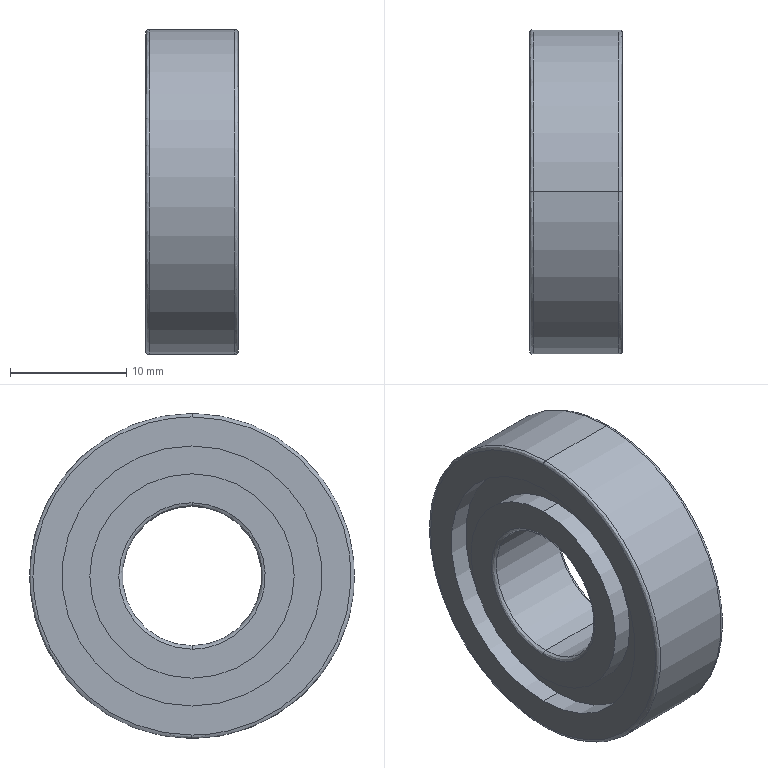Part | SolidWorks | features BaseBody 1 | 1 solid | 26 faces | box 8 x 28 x 28 mm | volume 3486 mm3 | cylinder 12 | spline 8 | plane 6 | commonest cylinder face diameters 17.6 x4 22.4 x4 12 x2 28 x2
STEP:
#1=CARTESIAN_POINT('',(0.,0.,13.7));
#2=VERTEX_POINT('',#1);
#3=CARTESIAN_POINT('',(0.,0.,-13.7));
#4=VERTEX_POINT('',#3);
#5=CARTESIAN_POINT('',(0.,0.,13.7));
#6=CARTESIAN_POINT('',(0.,-27.4,13.7));
#7=CARTESIAN_POINT('',(0.,-27.4,-13.7));
#8=CARTESIAN_POINT('',(0.,0.,-13.7));
#9=(BOUNDED_CURVE()B_SPLINE_CURVE(3,(#5,#6,#7,#8),.UNSPECIFIED.,.F.,.F.)B_SPLINE_CURVE_WITH_KNOTS((4,4),(0.,1.),.UNSPECIFIED.)CURVE()GEOMETRIC_REPRESENTATION_ITEM()RATIONAL_B_SPLINE_CURVE((1.,0.3333,0.3333,1.))REPRESENTATION_ITEM(''));
#10=EDGE_CURVE('',#2,#4,#9,.T.);
#11=ORIENTED_EDGE('',*,*,#10,.T.);
#12=CARTESIAN_POINT('',(0.3,0.,-14.));
#13=VERTEX_POINT('',#12);
#14=CARTESIAN_POINT('',(0.3,0.,-13.7));
#15=DIRECTION('',(0.,-1.,0.));
#16=DIRECTION('',(0.,0.,-1.));
#17=AXIS2_PLACEMENT_3D('',#14,#15,#16);
#18=CIRCLE('',#17,0.3);
#19=EDGE_CURVE('',#4,#13,#18,.T.);
#20=ORIENTED_EDGE('',*,*,#19,.T.);
#21=CARTESIAN_POINT('',(0.3,0.,14.));
#22=VERTEX_POINT('',#21);
#23=CARTESIAN_POINT('',(0.3,0.,0.));
#24=DIRECTION('',(1.,0.,0.));
#25=DIRECTION('',(0.,0.,-1.));
#26=AXIS2_PLACEMENT_3D('',#23,#24,#25);
#27=CIRCLE('',#26,14.);
#28=EDGE_CURVE('',#22,#13,#27,.T.);
#29=ORIENTED_EDGE('',*,*,#28,.F.);
#30=CARTESIAN_POINT('',(0.3,0.,13.7));
#31=DIRECTION('',(0.,1.,0.));
#32=DIRECTION('',(0.,0.,1.));
#33=AXIS2_PLACEMENT_3D('',#30,#31,#32);
#34=CIRCLE('',#33,0.3);
#35=EDGE_CURVE('',#2,#22,#34,.T.);
#36=ORIENTED_EDGE('',*,*,#35,.F.);
#37=EDGE_LOOP('',(#11,#20,#29,#36));
#38=FACE_OUTER_BOUND('',#37,.T.);
#39=CARTESIAN_POINT('',(0.,0.,-13.7));
#40=CARTESIAN_POINT('',(0.,-27.4,-13.7));
#41=CARTESIAN_POINT('',(0.,-27.4,13.7));
#42=CARTESIAN_POINT('',(0.,0.,13.7));
#43=CARTESIAN_POINT('',(0.,0.,-13.876));
#44=CARTESIAN_POINT('',(0.,-27.751,-13.876));
#45=CARTESIAN_POINT('',(0.,-27.751,13.876));
#46=CARTESIAN_POINT('',(0.,0.,13.876));
#47=CARTESIAN_POINT('',(0.1243,0.,-14.));
#48=CARTESIAN_POINT('',(0.1243,-28.,-14.));
#49=CARTESIAN_POINT('',(0.1243,-28.,14.));
#50=CARTESIAN_POINT('',(0.1243,0.,14.));
#51=CARTESIAN_POINT('',(0.3,0.,-14.));
#52=CARTESIAN_POINT('',(0.3,-28.,-14.));
#53=CARTESIAN_POINT('',(0.3,-28.,14.));
#54=CARTESIAN_POINT('',(0.3,0.,14.));
#55=(BOUNDED_SURFACE()B_SPLINE_SURFACE(3,3,((#39,#40,#41,#42),(#43,#44,#45,#46),(#47,#48,#49,#50),(#51,#52,#53,#54)),.UNSPECIFIED.,.F.,.F.,.F.)B_SPLINE_SURFACE_WITH_KNOTS((4,4),(4,4),(0.,1.),(0.,1.),.UNSPECIFIED.)GEOMETRIC_REPRESENTATION_ITEM()RATIONAL_B_SPLINE_SURFACE(((1.,0.3333,0.3333,1.),(0.8047,0.2682,0.2682,0.8047),(0.8047,0.2682,0.2682,0.8047),(1.,0.3333,0.3333,1.)))REPRESENTATION_ITEM('')SURFACE());
#56=ADVANCED_FACE('',(#38),#55,.T.);
#57=CARTESIAN_POINT('',(7.7,0.,-14.));
#58=VERTEX_POINT('',#57);
#59=CARTESIAN_POINT('',(7.7,0.,14.));
#60=VERTEX_POINT('',#59);
#61=CARTESIAN_POINT('',(7.7,0.,0.));
#62=DIRECTION('',(-1.,0.,0.));
#63=DIRECTION('',(0.,0.,-1.));
#64=AXIS2_PLACEMENT_3D('',#61,#62,#63);
#65=CIRCLE('',#64,14.);
#66=EDGE_CURVE('',#58,#60,#65,.T.);
#67=ORIENTED_EDGE('',*,*,#66,.F.);
#68=CARTESIAN_POINT('',(8.,0.,-13.7));
#69=VERTEX_POINT('',#68);
#70=CARTESIAN_POINT('',(7.7,0.,-13.7));
#71=DIRECTION('',(0.,-1.,0.));
#72=DIRECTION('',(0.,0.,-1.));
#73=AXIS2_PLACEMENT_3D('',#70,#71,#72);
#74=CIRCLE('',#73,0.3);
#75=EDGE_CURVE('',#58,#69,#74,.T.);
#76=ORIENTED_EDGE('',*,*,#75,.T.);
#77=CARTESIAN_POINT('',(8.,0.,13.7));
#78=VERTEX_POINT('',#77);
#79=CARTESIAN_POINT('',(8.,0.,-13.7));
#80=CARTESIAN_POINT('',(8.,-27.4,-13.7));
#81=CARTESIAN_POINT('',(8.,-27.4,13.7));
#82=CARTESIAN_POINT('',(8.,0.,13.7));
#83=(BOUNDED_CURVE()B_SPLINE_CURVE(3,(#79,#80,#81,#82),.UNSPECIFIED.,.F.,.F.)B_SPLINE_CURVE_WITH_KNOTS((4,4),(0.,1.),.UNSPECIFIED.)CURVE()GEOMETRIC_REPRESENTATION_ITEM()RATIONAL_B_SPLINE_CURVE((1.,0.3333,0.3333,1.))REPRESENTATION_ITEM(''));
#84=EDGE_CURVE('',#69,#78,#83,.T.);
#85=ORIENTED_EDGE('',*,*,#84,.T.);
#86=CARTESIAN_POINT('',(7.7,0.,13.7));
#87=DIRECTION('',(0.,1.,0.));
#88=DIRECTION('',(0.,0.,1.));
#89=AXIS2_PLACEMENT_3D('',#86,#87,#88);
#90=CIRCLE('',#89,0.3);
#91=EDGE_CURVE('',#60,#78,#90,.T.);
#92=ORIENTED_EDGE('',*,*,#91,.F.);
#93=EDGE_LOOP('',(#67,#76,#85,#92));
#94=FACE_OUTER_BOUND('',#93,.T.);
#95=CARTESIAN_POINT('',(7.7,0.,-14.));
#96=CARTESIAN_POINT('',(7.7,-28.,-14.));
#97=CARTESIAN_POINT('',(7.7,-28.,14.));
#98=CARTESIAN_POINT('',(7.7,0.,14.));
#99=CARTESIAN_POINT('',(7.876,0.,-14.));
#100=CARTESIAN_POINT('',(7.876,-28.,-14.));
#101=CARTESIAN_POINT('',(7.876,-28.,14.));
#102=CARTESIAN_POINT('',(7.876,0.,14.));
#103=CARTESIAN_POINT('',(8.,0.,-13.876));
#104=CARTESIAN_POINT('',(8.,-27.751,-13.876));
#105=CARTESIAN_POINT('',(8.,-27.751,13.876));
#106=CARTESIAN_POINT('',(8.,0.,13.876));
#107=CARTESIAN_POINT('',(8.,0.,-13.7));
#108=CARTESIAN_POINT('',(8.,-27.4,-13.7));
#109=CARTESIAN_POINT('',(8.,-27.4,13.7));
#110=CARTESIAN_POINT('',(8.,0.,13.7));
#111=(BOUNDED_SURFACE()B_SPLINE_SURFACE(3,3,((#95,#96,#97,#98),(#99,#100,#101,#102),(#103,#104,#105,#106),(#107,#108,#109,#110)),.UNSPECIFIED.,.F.,.F.,.F.)B_SPLINE_SURFACE_WITH_KNOTS((4,4),(4,4),(0.,1.),(0.,1.),.UNSPECIFIED.)GEOMETRIC_REPRESENTATION_ITEM()RATIONAL_B_SPLINE_SURFACE(((1.,0.3333,0.3333,1.),(0.8047,0.2682,0.2682,0.8047),(0.8047,0.2682,0.2682,0.8047),(1.,0.3333,0.3333,1.)))REPRESENTATION_ITEM('')SURFACE());
#112=ADVANCED_FACE('',(#94),#111,.T.);
#113=CARTESIAN_POINT('',(0.3,0.,6.));
#114=VERTEX_POINT('',#113);
#115=CARTESIAN_POINT('',(0.3,0.,-6.));
#116=VERTEX_POINT('',#115);
#117=CARTESIAN_POINT('',(0.3,0.,0.));
#118=DIRECTION('',(1.,0.,0.));
#119=DIRECTION('',(0.,0.,1.));
#120=AXIS2_PLACEMENT_3D('',#117,#118,#119);
#121=CIRCLE('',#120,6.);
#122=EDGE_CURVE('',#114,#116,#121,.T.);
#123=ORIENTED_EDGE('',*,*,#122,.T.);
#124=CARTESIAN_POINT('',(0.,0.,-6.3));
#125=VERTEX_POINT('',#124);
#126=CARTESIAN_POINT('',(0.3,0.,-6.3));
#127=DIRECTION('',(0.,-1.,0.));
#128=DIRECTION('',(0.,0.,-1.));
#129=AXIS2_PLACEMENT_3D('',#126,#127,#128);
#130=CIRCLE('',#129,0.3);
#131=EDGE_CURVE('',#116,#125,#130,.T.);
#132=ORIENTED_EDGE('',*,*,#131,.T.);
#133=CARTESIAN_POINT('',(0.,0.,6.3));
#134=VERTEX_POINT('',#133);
#135=CARTESIAN_POINT('',(0.,0.,6.3));
#136=CARTESIAN_POINT('',(0.,-0.1928,6.3));
#137=CARTESIAN_POINT('',(0.,-0.4806,6.287));
#138=CARTESIAN_POINT('',(0.,-0.8142,6.248));
#139=CARTESIAN_POINT('',(0.,-0.9805,6.224));
#140=CARTESIAN_POINT('',(0.,-1.052,6.212));
#141=CARTESIAN_POINT('',(0.,-1.099,6.203));
#142=CARTESIAN_POINT('',(0.,-1.121,6.199));
#143=CARTESIAN_POINT('',(0.,-1.347,6.158));
#144=CARTESIAN_POINT('',(0.,-1.644,6.088));
#145=CARTESIAN_POINT('',(0.,-1.984,5.981));
#146=CARTESIAN_POINT('',(0.,-2.128,5.93));
#147=CARTESIAN_POINT('',(0.,-2.224,5.895));
#148=CARTESIAN_POINT('',(0.,-2.27,5.877));
#149=CARTESIAN_POINT('',(0.,-2.517,5.779));
#150=CARTESIAN_POINT('',(0.,-2.806,5.648));
#151=CARTESIAN_POINT('',(0.,-3.085,5.494));
#152=CARTESIAN_POINT('',(0.,-3.268,5.387));
#153=CARTESIAN_POINT('',(0.,-3.356,5.333));
#154=CARTESIAN_POINT('',(0.,-3.811,5.035));
#155=CARTESIAN_POINT('',(0.,-4.147,4.762));
#156=CARTESIAN_POINT('',(0.,-4.608,4.301));
#157=CARTESIAN_POINT('',(0.,-4.826,4.06));
#158=CARTESIAN_POINT('',(0.,-5.057,3.76));
#159=CARTESIAN_POINT('',(0.,-5.151,3.627));
#160=CARTESIAN_POINT('',(0.,-5.213,3.538));
#161=CARTESIAN_POINT('',(0.,-5.244,3.492));
#162=CARTESIAN_POINT('',(0.,-5.389,3.269));
#163=CARTESIAN_POINT('',(0.,-5.55,2.995));
#164=CARTESIAN_POINT('',(0.,-5.712,2.661));
#165=CARTESIAN_POINT('',(0.,-5.776,2.516));
#166=CARTESIAN_POINT('',(0.,-5.818,2.418));
#167=CARTESIAN_POINT('',(0.,-5.839,2.366));
#168=CARTESIAN_POINT('',(0.,-5.933,2.129));
#169=CARTESIAN_POINT('',(0.,-6.031,1.84));
#170=CARTESIAN_POINT('',(0.,-6.121,1.496));
#171=CARTESIAN_POINT('',(0.,-6.16,1.322));
#172=CARTESIAN_POINT('',(0.,-6.175,1.247));
#173=CARTESIAN_POINT('',(0.,-6.185,1.197));
#174=CARTESIAN_POINT('',(0.,-6.19,1.17));
#175=CARTESIAN_POINT('',(0.,-6.265,0.7678));
#176=CARTESIAN_POINT('',(0.,-6.3,0.385));
#177=CARTESIAN_POINT('',(0.,-6.3,-0.1925));
#178=CARTESIAN_POINT('',(0.,-6.287,-0.4802));
#179=CARTESIAN_POINT('',(0.,-6.249,-0.8139));
#180=CARTESIAN_POINT('',(0.,-6.224,-0.9803));
#181=CARTESIAN_POINT('',(0.,-6.212,-1.051));
#182=CARTESIAN_POINT('',(0.,-6.203,-1.099));
#183=CARTESIAN_POINT('',(0.,-6.199,-1.121));
#184=CARTESIAN_POINT('',(0.,-6.158,-1.347));
#185=CARTESIAN_POINT('',(0.,-6.088,-1.644));
#186=CARTESIAN_POINT('',(0.,-5.981,-1.984));
#187=CARTESIAN_POINT('',(0.,-5.93,-2.128));
#188=CARTESIAN_POINT('',(0.,-5.895,-2.224));
#189=CARTESIAN_POINT('',(0.,-5.877,-2.27));
#190=CARTESIAN_POINT('',(0.,-5.779,-2.517));
#191=CARTESIAN_POINT('',(0.,-5.648,-2.806));
#192=CARTESIAN_POINT('',(0.,-5.494,-3.085));
#193=CARTESIAN_POINT('',(0.,-5.387,-3.268));
#194=CARTESIAN_POINT('',(0.,-5.333,-3.356));
#195=CARTESIAN_POINT('',(0.,-5.035,-3.811));
#196=CARTESIAN_POINT('',(0.,-4.762,-4.147));
#197=CARTESIAN_POINT('',(0.,-4.301,-4.608));
#198=CARTESIAN_POINT('',(0.,-4.06,-4.826));
#199=CARTESIAN_POINT('',(0.,-3.76,-5.057));
#200=CARTESIAN_POINT('',(0.,-3.627,-5.151));
#201=CARTESIAN_POINT('',(0.,-3.538,-5.213));
#202=CARTESIAN_POINT('',(0.,-3.492,-5.244));
#203=CARTESIAN_POINT('',(0.,-3.269,-5.389));
#204=CARTESIAN_POINT('',(0.,-2.995,-5.55));
#205=CARTESIAN_POINT('',(0.,-2.661,-5.712));
#206=CARTESIAN_POINT('',(0.,-2.516,-5.776));
#207=CARTESIAN_POINT('',(0.,-2.418,-5.818));
#208=CARTESIAN_POINT('',(0.,-2.366,-5.839));
#209=CARTESIAN_POINT('',(0.,-2.129,-5.933));
#210=CARTESIAN_POINT('',(0.,-1.84,-6.031));
#211=CARTESIAN_POINT('',(0.,-1.496,-6.121));
#212=CARTESIAN_POINT('',(0.,-1.322,-6.16));
#213=CARTESIAN_POINT('',(0.,-1.247,-6.175));
#214=CARTESIAN_POINT('',(0.,-1.197,-6.185));
#215=CARTESIAN_POINT('',(0.,-1.17,-6.19));
#216=CARTESIAN_POINT('',(0.,-0.768,-6.265));
#217=CARTESIAN_POINT('',(0.,-0.3859,-6.3));
#218=CARTESIAN_POINT('',(0.,0.,-6.3));
#219=B_SPLINE_CURVE_WITH_KNOTS('',3,(#135,#136,#137,#138,#139,#140,#141,#142,#143,#144,#145,#146,#147,#148,#149,#150,#151,#152,#153,#154,#155,#156,#157,#158,#159,#160,#161,#162,#163,#164,#165,#166,#167,#168,#169,#170,#171,#172,#173,#174,#175,#176,#177,#178,#179,#180,#181,#182,#183,#184,#185,#186,#187,#188,#189,#190,#191,#192,#193,#194,#195,#196,#197,#198,#199,#200,#201,#202,#203,#204,#205,#206,#207,#208,#209,#210,#211,#212,#213,#214,#215,#216,#217,#218),.UNSPECIFIED.,.F.,.F.,(4,1,1,1,2,2,1,1,2,2,1,2,2,2,1,1,2,2,1,1,2,2,1,1,1,2,2,2,1,1,1,2,2,1,1,2,2,1,2,2,2,1,1,2,2,1,1,2,2,1,1,1,2,2,4),(0.,0.03125,0.04688,0.05469,0.05859,0.0625,0.09375,0.1094,0.1172,0.125,0.1563,0.1719,0.1875,0.25,0.2813,0.2969,0.3047,0.3125,0.3438,0.3594,0.3672,0.375,0.4063,0.4219,0.4297,0.4336,0.4375,0.5,0.5312,0.5469,0.5547,0.5586,0.5625,0.5937,0.6094,0.6172,0.625,0.6562,0.6719,0.6875,0.75,0.7812,0.7969,0.8047,0.8125,0.8437,0.8594,0.8672,0.875,0.9062,0.9219,0.9297,0.9336,0.9375,1.),.UNSPECIFIED.);
#220=EDGE_CURVE('',#134,#125,#219,.T.);
#221=ORIENTED_EDGE('',*,*,#220,.F.);
#222=CARTESIAN_POINT('',(0.3,0.,6.3));
#223=DIRECTION('',(0.,1.,0.));
#224=DIRECTION('',(0.,0.,1.));
#225=AXIS2_PLACEMENT_3D('',#222,#223,#224);
#226=CIRCLE('',#225,0.3);
#227=EDGE_CURVE('',#114,#134,#226,.T.);
#228=ORIENTED_EDGE('',*,*,#227,.F.);
#229=EDGE_LOOP('',(#123,#132,#221,#228));
#230=FACE_OUTER_BOUND('',#229,.T.);
#231=CARTESIAN_POINT('',(0.3,0.,-6.));
#232=CARTESIAN_POINT('',(0.3,-12.,-6.));
#233=CARTESIAN_POINT('',(0.3,-12.,6.));
#234=CARTESIAN_POINT('',(0.3,0.,6.));
#235=CARTESIAN_POINT('',(0.1243,0.,-6.));
#236=CARTESIAN_POINT('',(0.1243,-12.,-6.));
#237=CARTESIAN_POINT('',(0.1243,-12.,6.));
#238=CARTESIAN_POINT('',(0.1243,0.,6.));
#239=CARTESIAN_POINT('',(0.,0.,-6.124));
#240=CARTESIAN_POINT('',(0.,-12.249,-6.124));
#241=CARTESIAN_POINT('',(0.,-12.249,6.124));
#242=CARTESIAN_POINT('',(0.,0.,6.124));
#243=CARTESIAN_POINT('',(0.,0.,-6.3));
#244=CARTESIAN_POINT('',(0.,-12.6,-6.3));
#245=CARTESIAN_POINT('',(0.,-12.6,6.3));
#246=CARTESIAN_POINT('',(0.,0.,6.3));
#247=(BOUNDED_SURFACE()B_SPLINE_SURFACE(3,3,((#231,#232,#233,#234),(#235,#236,#237,#238),(#239,#240,#241,#242),(#243,#244,#245,#246)),.UNSPECIFIED.,.F.,.F.,.F.)B_SPLINE_SURFACE_WITH_KNOTS((4,4),(4,4),(0.,1.),(0.,1.),.UNSPECIFIED.)GEOMETRIC_REPRESENTATION_ITEM()RATIONAL_B_SPLINE_SURFACE(((1.,0.3333,0.3333,1.),(0.8047,0.2682,0.2682,0.8047),(0.8047,0.2682,0.2682,0.8047),(1.,0.3333,0.3333,1.)))REPRESENTATION_ITEM('')SURFACE());
#248=ADVANCED_FACE('',(#230),#247,.T.);
#249=CARTESIAN_POINT('',(8.,0.,-6.3));
#250=VERTEX_POINT('',#249);
#251=CARTESIAN_POINT('',(8.,0.,6.3));
#252=VERTEX_POINT('',#251);
#253=CARTESIAN_POINT('',(8.,0.,-6.3));
#254=CARTESIAN_POINT('',(8.,-0.1928,-6.3));
#255=CARTESIAN_POINT('',(8.,-0.4806,-6.287));
#256=CARTESIAN_POINT('',(8.,-0.8142,-6.248));
#257=CARTESIAN_POINT('',(8.,-0.9805,-6.224));
#258=CARTESIAN_POINT('',(8.,-1.052,-6.212));
#259=CARTESIAN_POINT('',(8.,-1.099,-6.203));
#260=CARTESIAN_POINT('',(8.,-1.121,-6.199));
#261=CARTESIAN_POINT('',(8.,-1.347,-6.158));
#262=CARTESIAN_POINT('',(8.,-1.644,-6.088));
#263=CARTESIAN_POINT('',(8.,-1.984,-5.981));
#264=CARTESIAN_POINT('',(8.,-2.128,-5.93));
#265=CARTESIAN_POINT('',(8.,-2.224,-5.895));
#266=CARTESIAN_POINT('',(8.,-2.27,-5.877));
#267=CARTESIAN_POINT('',(8.,-2.517,-5.779));
#268=CARTESIAN_POINT('',(8.,-2.806,-5.648));
#269=CARTESIAN_POINT('',(8.,-3.085,-5.494));
#270=CARTESIAN_POINT('',(8.,-3.268,-5.387));
#271=CARTESIAN_POINT('',(8.,-3.356,-5.333));
#272=CARTESIAN_POINT('',(8.,-3.811,-5.035));
#273=CARTESIAN_POINT('',(8.,-4.147,-4.762));
#274=CARTESIAN_POINT('',(8.,-4.608,-4.301));
#275=CARTESIAN_POINT('',(8.,-4.826,-4.06));
#276=CARTESIAN_POINT('',(8.,-5.057,-3.76));
#277=CARTESIAN_POINT('',(8.,-5.151,-3.627));
#278=CARTESIAN_POINT('',(8.,-5.213,-3.538));
#279=CARTESIAN_POINT('',(8.,-5.244,-3.492));
#280=CARTESIAN_POINT('',(8.,-5.389,-3.269));
#281=CARTESIAN_POINT('',(8.,-5.55,-2.995));
#282=CARTESIAN_POINT('',(8.,-5.712,-2.661));
#283=CARTESIAN_POINT('',(8.,-5.776,-2.516));
#284=CARTESIAN_POINT('',(8.,-5.818,-2.418));
#285=CARTESIAN_POINT('',(8.,-5.839,-2.366));
#286=CARTESIAN_POINT('',(8.,-5.933,-2.129));
#287=CARTESIAN_POINT('',(8.,-6.031,-1.84));
#288=CARTESIAN_POINT('',(8.,-6.121,-1.496));
#289=CARTESIAN_POINT('',(8.,-6.16,-1.322));
#290=CARTESIAN_POINT('',(8.,-6.175,-1.247));
#291=CARTESIAN_POINT('',(8.,-6.185,-1.197));
#292=CARTESIAN_POINT('',(8.,-6.19,-1.17));
#293=CARTESIAN_POINT('',(8.,-6.265,-0.7678));
#294=CARTESIAN_POINT('',(8.,-6.3,-0.385));
#295=CARTESIAN_POINT('',(8.,-6.3,0.1925));
#296=CARTESIAN_POINT('',(8.,-6.287,0.4802));
#297=CARTESIAN_POINT('',(8.,-6.249,0.8139));
#298=CARTESIAN_POINT('',(8.,-6.224,0.9803));
#299=CARTESIAN_POINT('',(8.,-6.212,1.051));
#300=CARTESIAN_POINT('',(8.,-6.203,1.099));
#301=CARTESIAN_POINT('',(8.,-6.199,1.121));
#302=CARTESIAN_POINT('',(8.,-6.158,1.347));
#303=CARTESIAN_POINT('',(8.,-6.088,1.644));
#304=CARTESIAN_POINT('',(8.,-5.981,1.984));
#305=CARTESIAN_POINT('',(8.,-5.93,2.128));
#306=CARTESIAN_POINT('',(8.,-5.895,2.224));
#307=CARTESIAN_POINT('',(8.,-5.877,2.27));
#308=CARTESIAN_POINT('',(8.,-5.779,2.517));
#309=CARTESIAN_POINT('',(8.,-5.648,2.806));
#310=CARTESIAN_POINT('',(8.,-5.494,3.085));
#311=CARTESIAN_POINT('',(8.,-5.387,3.268));
#312=CARTESIAN_POINT('',(8.,-5.333,3.356));
#313=CARTESIAN_POINT('',(8.,-5.035,3.811));
#314=CARTESIAN_POINT('',(8.,-4.762,4.147));
#315=CARTESIAN_POINT('',(8.,-4.301,4.608));
#316=CARTESIAN_POINT('',(8.,-4.06,4.826));
#317=CARTESIAN_POINT('',(8.,-3.76,5.057));
#318=CARTESIAN_POINT('',(8.,-3.627,5.151));
#319=CARTESIAN_POINT('',(8.,-3.538,5.213));
#320=CARTESIAN_POINT('',(8.,-3.492,5.244));
#321=CARTESIAN_POINT('',(8.,-3.269,5.389));
#322=CARTESIAN_POINT('',(8.,-2.995,5.55));
#323=CARTESIAN_POINT('',(8.,-2.661,5.712));
#324=CARTESIAN_POINT('',(8.,-2.516,5.776));
#325=CARTESIAN_POINT('',(8.,-2.418,5.818));
#326=CARTESIAN_POINT('',(8.,-2.366,5.839));
#327=CARTESIAN_POINT('',(8.,-2.129,5.933));
#328=CARTESIAN_POINT('',(8.,-1.84,6.031));
#329=CARTESIAN_POINT('',(8.,-1.496,6.121));
#330=CARTESIAN_POINT('',(8.,-1.322,6.16));
#331=CARTESIAN_POINT('',(8.,-1.247,6.175));
#332=CARTESIAN_POINT('',(8.,-1.197,6.185));
#333=CARTESIAN_POINT('',(8.,-1.17,6.19));
#334=CARTESIAN_POINT('',(8.,-0.768,6.265));
#335=CARTESIAN_POINT('',(8.,-0.3859,6.3));
#336=CARTESIAN_POINT('',(8.,0.,6.3));
#337=B_SPLINE_CURVE_WITH_KNOTS('',3,(#253,#254,#255,#256,#257,#258,#259,#260,#261,#262,#263,#264,#265,#266,#267,#268,#269,#270,#271,#272,#273,#274,#275,#276,#277,#278,#279,#280,#281,#282,#283,#284,#285,#286,#287,#288,#289,#290,#291,#292,#293,#294,#295,#296,#297,#298,#299,#300,#301,#302,#303,#304,#305,#306,#307,#308,#309,#310,#311,#312,#313,#314,#315,#316,#317,#318,#319,#320,#321,#322,#323,#324,#325,#326,#327,#328,#329,#330,#331,#332,#333,#334,#335,#336),.UNSPECIFIED.,.F.,.F.,(4,1,1,1,2,2,1,1,2,2,1,2,2,2,1,1,2,2,1,1,2,2,1,1,1,2,2,2,1,1,1,2,2,1,1,2,2,1,2,2,2,1,1,2,2,1,1,2,2,1,1,1,2,2,4),(0.,0.03125,0.04688,0.05469,0.05859,0.0625,0.09375,0.1094,0.1172,0.125,0.1563,0.1719,0.1875,0.25,0.2813,0.2969,0.3047,0.3125,0.3438,0.3594,0.3672,0.375,0.4063,0.4219,0.4297,0.4336,0.4375,0.5,0.5313,0.5469,0.5547,0.5586,0.5625,0.5938,0.6094,0.6172,0.625,0.6563,0.6719,0.6875,0.75,0.7813,0.7969,0.8047,0.8125,0.8438,0.8594,0.8672,0.875,0.9063,0.9219,0.9297,0.9336,0.9375,1.),.UNSPECIFIED.);
#338=EDGE_CURVE('',#250,#252,#337,.T.);
#339=ORIENTED_EDGE('',*,*,#338,.F.);
#340=CARTESIAN_POINT('',(7.7,0.,-6.));
#341=VERTEX_POINT('',#340);
#342=CARTESIAN_POINT('',(7.7,0.,-6.3));
#343=DIRECTION('',(0.,-1.,0.));
#344=DIRECTION('',(0.,0.,-1.));
#345=AXIS2_PLACEMENT_3D('',#342,#343,#344);
#346=CIRCLE('',#345,0.3);
#347=EDGE_CURVE('',#250,#341,#346,.T.);
#348=ORIENTED_EDGE('',*,*,#347,.T.);
#349=CARTESIAN_POINT('',(7.7,0.,6.));
#350=VERTEX_POINT('',#349);
#351=CARTESIAN_POINT('',(7.7,0.,0.));
#352=DIRECTION('',(-1.,0.,0.));
#353=DIRECTION('',(0.,0.,1.));
#354=AXIS2_PLACEMENT_3D('',#351,#352,#353);
#355=CIRCLE('',#354,6.);
#356=EDGE_CURVE('',#341,#350,#355,.T.);
#357=ORIENTED_EDGE('',*,*,#356,.T.);
#358=CARTESIAN_POINT('',(7.7,0.,6.3));
#359=DIRECTION('',(0.,1.,0.));
#360=DIRECTION('',(0.,0.,1.));
#361=AXIS2_PLACEMENT_3D('',#358,#359,#360);
#362=CIRCLE('',#361,0.3);
#363=EDGE_CURVE('',#252,#350,#362,.T.);
#364=ORIENTED_EDGE('',*,*,#363,.F.);
#365=EDGE_LOOP('',(#339,#348,#357,#364));
#366=FACE_OUTER_BOUND('',#365,.T.);
#367=CARTESIAN_POINT('',(8.,0.,-6.3));
#368=CARTESIAN_POINT('',(8.,-12.6,-6.3));
#369=CARTESIAN_POINT('',(8.,-12.6,6.3));
#370=CARTESIAN_POINT('',(8.,0.,6.3));
#371=CARTESIAN_POINT('',(8.,0.,-6.124));
#372=CARTESIAN_POINT('',(8.,-12.249,-6.124));
#373=CARTESIAN_POINT('',(8.,-12.249,6.124));
#374=CARTESIAN_POINT('',(8.,0.,6.124));
#375=CARTESIAN_POINT('',(7.876,0.,-6.));
#376=CARTESIAN_POINT('',(7.876,-12.,-6.));
#377=CARTESIAN_POINT('',(7.876,-12.,6.));
#378=CARTESIAN_POINT('',(7.876,0.,6.));
#379=CARTESIAN_POINT('',(7.7,0.,-6.));
#380=CARTESIAN_POINT('',(7.7,-12.,-6.));
#381=CARTESIAN_POINT('',(7.7,-12.,6.));
#382=CARTESIAN_POINT('',(7.7,0.,6.));
#383=(BOUNDED_SURFACE()B_SPLINE_SURFACE(3,3,((#367,#368,#369,#370),(#371,#372,#373,#374),(#375,#376,#377,#378),(#379,#380,#381,#382)),.UNSPECIFIED.,.F.,.F.,.T.)B_SPLINE_SURFACE_WITH_KNOTS((4,4),(4,4),(0.,1.),(0.,1.),.UNSPECIFIED.)GEOMETRIC_REPRESENTATION_ITEM()RATIONAL_B_SPLINE_SURFACE(((1.,0.3333,0.3333,1.),(0.8047,0.2682,0.2682,0.8047),(0.8047,0.2682,0.2682,0.8047),(1.,0.3333,0.3333,1.)))REPRESENTATION_ITEM('')SURFACE());
#384=ADVANCED_FACE('',(#366),#383,.T.);
#385=CARTESIAN_POINT('',(0.3,0.,0.));
#386=DIRECTION('',(1.,0.,0.));
#387=DIRECTION('',(0.,0.,-1.));
#388=AXIS2_PLACEMENT_3D('',#385,#386,#387);
#389=CIRCLE('',#388,14.);
#390=EDGE_CURVE('',#13,#22,#389,.T.);
#391=ORIENTED_EDGE('',*,*,#390,.T.);
#392=CARTESIAN_POINT('',(4.,0.,14.));
#393=DIRECTION('',(1.,0.,0.));
#394=VECTOR('',#393,1000.);
#395=LINE('',#392,#394);
#396=EDGE_CURVE('',#22,#60,#395,.T.);
#397=ORIENTED_EDGE('',*,*,#396,.T.);
#398=CARTESIAN_POINT('',(7.7,0.,0.));
#399=DIRECTION('',(-1.,0.,0.));
#400=DIRECTION('',(0.,0.,-1.));
#401=AXIS2_PLACEMENT_3D('',#398,#399,#400);
#402=CIRCLE('',#401,14.);
#403=EDGE_CURVE('',#60,#58,#402,.T.);
#404=ORIENTED_EDGE('',*,*,#403,.T.);
#405=CARTESIAN_POINT('',(4.,0.,-14.));
#406=DIRECTION('',(1.,0.,0.));
#407=VECTOR('',#406,1000.);
#408=LINE('',#405,#407);
#409=EDGE_CURVE('',#13,#58,#408,.T.);
#410=ORIENTED_EDGE('',*,*,#409,.F.);
#411=EDGE_LOOP('',(#391,#397,#404,#410));
#412=FACE_OUTER_BOUND('',#411,.T.);
#413=CARTESIAN_POINT('',(4.,0.,0.));
#414=DIRECTION('',(1.,0.,0.));
#415=DIRECTION('',(0.,0.,-1.));
#416=AXIS2_PLACEMENT_3D('',#413,#414,#415);
#417=CYLINDRICAL_SURFACE('',#416,14.);
#418=ADVANCED_FACE('',(#412),#417,.T.);
#419=CARTESIAN_POINT('',(0.,0.,11.2));
#420=VERTEX_POINT('',#419);
#421=CARTESIAN_POINT('',(0.,0.,-11.2));
#422=VERTEX_POINT('',#421);
#423=CARTESIAN_POINT('',(0.,0.,0.));
#424=DIRECTION('',(1.,0.,0.));
#425=DIRECTION('',(0.,0.,-1.));
#426=AXIS2_PLACEMENT_3D('',#423,#424,#425);
#427=CIRCLE('',#426,11.2);
#428=EDGE_CURVE('',#420,#422,#427,.T.);
#429=ORIENTED_EDGE('',*,*,#428,.F.);
#430=CARTESIAN_POINT('',(1.76,0.,11.2));
#431=VERTEX_POINT('',#430);
#432=CARTESIAN_POINT('',(0.88,0.,11.2));
#433=DIRECTION('',(1.,0.,0.));
#434=VECTOR('',#433,1000.);
#435=LINE('',#432,#434);
#436=EDGE_CURVE('',#420,#431,#435,.T.);
#437=ORIENTED_EDGE('',*,*,#436,.T.);
#438=CARTESIAN_POINT('',(1.76,0.,-11.2));
#439=VERTEX_POINT('',#438);
#440=CARTESIAN_POINT('',(1.76,0.,0.));
#441=DIRECTION('',(-1.,0.,0.));
#442=DIRECTION('',(0.,0.,-1.));
#443=AXIS2_PLACEMENT_3D('',#440,#441,#442);
#444=CIRCLE('',#443,11.2);
#445=EDGE_CURVE('',#439,#431,#444,.T.);
#446=ORIENTED_EDGE('',*,*,#445,.F.);
#447=CARTESIAN_POINT('',(0.88,0.,-11.2));
#448=DIRECTION('',(1.,0.,0.));
#449=VECTOR('',#448,1000.);
#450=LINE('',#447,#449);
#451=EDGE_CURVE('',#422,#439,#450,.T.);
#452=ORIENTED_EDGE('',*,*,#451,.F.);
#453=EDGE_LOOP('',(#429,#437,#446,#452));
#454=FACE_OUTER_BOUND('',#453,.T.);
#455=CARTESIAN_POINT('',(0.88,0.,0.));
#456=DIRECTION('',(1.,0.,0.));
#457=DIRECTION('',(0.,0.,-1.));
#458=AXIS2_PLACEMENT_3D('',#455,#456,#457);
#459=CYLINDRICAL_SURFACE('',#458,11.2);
#460=ADVANCED_FACE('',(#454),#459,.F.);
#461=CARTESIAN_POINT('',(6.24,0.,11.2));
#462=VERTEX_POINT('',#461);
#463=CARTESIAN_POINT('',(6.24,0.,-11.2));
#464=VERTEX_POINT('',#463);
#465=CARTESIAN_POINT('',(6.24,0.,0.));
#466=DIRECTION('',(1.,0.,0.));
#467=DIRECTION('',(0.,0.,-1.));
#468=AXIS2_PLACEMENT_3D('',#465,#466,#467);
#469=CIRCLE('',#468,11.2);
#470=EDGE_CURVE('',#462,#464,#469,.T.);
#471=ORIENTED_EDGE('',*,*,#470,.F.);
#472=CARTESIAN_POINT('',(8.,0.,11.2));
#473=VERTEX_POINT('',#472);
#474=CARTESIAN_POINT('',(7.12,0.,11.2));
#475=DIRECTION('',(1.,0.,0.));
#476=VECTOR('',#475,1000.);
#477=LINE('',#474,#476);
#478=EDGE_CURVE('',#462,#473,#477,.T.);
#479=ORIENTED_EDGE('',*,*,#478,.T.);
#480=CARTESIAN_POINT('',(8.,0.,-11.2));
#481=VERTEX_POINT('',#480);
#482=CARTESIAN_POINT('',(8.,0.,0.));
#483=DIRECTION('',(-1.,0.,0.));
#484=DIRECTION('',(0.,0.,-1.));
#485=AXIS2_PLACEMENT_3D('',#482,#483,#484);
#486=CIRCLE('',#485,11.2);
#487=EDGE_CURVE('',#481,#473,#486,.T.);
#488=ORIENTED_EDGE('',*,*,#487,.F.);
#489=CARTESIAN_POINT('',(7.12,0.,-11.2));
#490=DIRECTION('',(1.,0.,0.));
#491=VECTOR('',#490,1000.);
#492=LINE('',#489,#491);
#493=EDGE_CURVE('',#464,#481,#492,.T.);
#494=ORIENTED_EDGE('',*,*,#493,.F.);
#495=EDGE_LOOP('',(#471,#479,#488,#494));
#496=FACE_OUTER_BOUND('',#495,.T.);
#497=CARTESIAN_POINT('',(7.12,0.,0.));
#498=DIRECTION('',(1.,0.,0.));
#499=DIRECTION('',(0.,0.,-1.));
#500=AXIS2_PLACEMENT_3D('',#497,#498,#499);
#501=CYLINDRICAL_SURFACE('',#500,11.2);
#502=ADVANCED_FACE('',(#496),#501,.F.);
#503=CARTESIAN_POINT('',(0.,0.,-8.8));
#504=VERTEX_POINT('',#503);
#505=CARTESIAN_POINT('',(0.,0.,8.8));
#506=VERTEX_POINT('',#505);
#507=CARTESIAN_POINT('',(0.,0.,0.));
#508=DIRECTION('',(1.,0.,0.));
#509=DIRECTION('',(0.,0.,-1.));
#510=AXIS2_PLACEMENT_3D('',#507,#508,#509);
#511=CIRCLE('',#510,8.8);
#512=EDGE_CURVE('',#504,#506,#511,.T.);
#513=ORIENTED_EDGE('',*,*,#512,.T.);
#514=CARTESIAN_POINT('',(1.76,0.,8.8));
#515=VERTEX_POINT('',#514);
#516=CARTESIAN_POINT('',(0.88,0.,8.8));
#517=DIRECTION('',(1.,0.,0.));
#518=VECTOR('',#517,1000.);
#519=LINE('',#516,#518);
#520=EDGE_CURVE('',#506,#515,#519,.T.);
#521=ORIENTED_EDGE('',*,*,#520,.T.);
#522=CARTESIAN_POINT('',(1.76,0.,-8.8));
#523=VERTEX_POINT('',#522);
#524=CARTESIAN_POINT('',(1.76,0.,0.));
#525=DIRECTION('',(1.,0.,0.));
#526=DIRECTION('',(0.,0.,-1.));
#527=AXIS2_PLACEMENT_3D('',#524,#525,#526);
#528=CIRCLE('',#527,8.8);
#529=EDGE_CURVE('',#523,#515,#528,.T.);
#530=ORIENTED_EDGE('',*,*,#529,.F.);
#531=CARTESIAN_POINT('',(0.88,0.,-8.8));
#532=DIRECTION('',(1.,0.,0.));
#533=VECTOR('',#532,1000.);
#534=LINE('',#531,#533);
#535=EDGE_CURVE('',#504,#523,#534,.T.);
#536=ORIENTED_EDGE('',*,*,#535,.F.);
#537=EDGE_LOOP('',(#513,#521,#530,#536));
#538=FACE_OUTER_BOUND('',#537,.T.);
#539=CARTESIAN_POINT('',(0.88,0.,0.));
#540=DIRECTION('',(1.,0.,0.));
#541=DIRECTION('',(0.,0.,-1.));
#542=AXIS2_PLACEMENT_3D('',#539,#540,#541);
#543=CYLINDRICAL_SURFACE('',#542,8.8);
#544=ADVANCED_FACE('',(#538),#543,.T.);
#545=CARTESIAN_POINT('',(6.24,0.,8.8));
#546=VERTEX_POINT('',#545);
#547=CARTESIAN_POINT('',(6.24,0.,-8.8));
#548=VERTEX_POINT('',#547);
#549=CARTESIAN_POINT('',(6.24,0.,0.));
#550=DIRECTION('',(-1.,0.,0.));
#551=DIRECTION('',(0.,0.,-1.));
#552=AXIS2_PLACEMENT_3D('',#549,#550,#551);
#553=CIRCLE('',#552,8.8);
#554=EDGE_CURVE('',#546,#548,#553,.T.);
#555=ORIENTED_EDGE('',*,*,#554,.F.);
#556=CARTESIAN_POINT('',(8.,0.,8.8));
#557=VERTEX_POINT('',#556);
#558=CARTESIAN_POINT('',(7.12,0.,8.8));
#559=DIRECTION('',(1.,0.,0.));
#560=VECTOR('',#559,1000.);
#561=LINE('',#558,#560);
#562=EDGE_CURVE('',#546,#557,#561,.T.);
#563=ORIENTED_EDGE('',*,*,#562,.T.);
#564=CARTESIAN_POINT('',(8.,0.,-8.8));
#565=VERTEX_POINT('',#564);
#566=CARTESIAN_POINT('',(8.,0.,0.));
#567=DIRECTION('',(-1.,0.,0.));
#568=DIRECTION('',(0.,0.,-1.));
#569=AXIS2_PLACEMENT_3D('',#566,#567,#568);
#570=CIRCLE('',#569,8.8);
#571=EDGE_CURVE('',#557,#565,#570,.T.);
#572=ORIENTED_EDGE('',*,*,#571,.T.);
#573=CARTESIAN_POINT('',(7.12,0.,-8.8));
#574=DIRECTION('',(1.,0.,0.));
#575=VECTOR('',#574,1000.);
#576=LINE('',#573,#575);
#577=EDGE_CURVE('',#548,#565,#576,.T.);
#578=ORIENTED_EDGE('',*,*,#577,.F.);
#579=EDGE_LOOP('',(#555,#563,#572,#578));
#580=FACE_OUTER_BOUND('',#579,.T.);
#581=CARTESIAN_POINT('',(7.12,0.,0.));
#582=DIRECTION('',(1.,0.,0.));
#583=DIRECTION('',(0.,0.,-1.));
#584=AXIS2_PLACEMENT_3D('',#581,#582,#583);
#585=CYLINDRICAL_SURFACE('',#584,8.8);
#586=ADVANCED_FACE('',(#580),#585,.T.);
#587=ORIENTED_EDGE('',*,*,#122,.F.);
#588=CARTESIAN_POINT('',(4.,0.,6.));
#589=DIRECTION('',(1.,0.,0.));
#590=VECTOR('',#589,1000.);
#591=LINE('',#588,#590);
#592=EDGE_CURVE('',#114,#350,#591,.T.);
#593=ORIENTED_EDGE('',*,*,#592,.T.);
#594=ORIENTED_EDGE('',*,*,#356,.F.);
#595=CARTESIAN_POINT('',(4.,0.,-6.));
#596=DIRECTION('',(1.,0.,0.));
#597=VECTOR('',#596,1000.);
#598=LINE('',#595,#597);
#599=EDGE_CURVE('',#116,#341,#598,.T.);
#600=ORIENTED_EDGE('',*,*,#599,.F.);
#601=EDGE_LOOP('',(#587,#593,#594,#600));
#602=FACE_OUTER_BOUND('',#601,.T.);
#603=CARTESIAN_POINT('',(4.,0.,0.));
#604=DIRECTION('',(1.,0.,0.));
#605=DIRECTION('',(0.,0.,-1.));
#606=AXIS2_PLACEMENT_3D('',#603,#604,#605);
#607=CYLINDRICAL_SURFACE('',#606,6.);
#608=ADVANCED_FACE('',(#602),#607,.F.);
#609=ORIENTED_EDGE('',*,*,#396,.F.);
#610=ORIENTED_EDGE('',*,*,#28,.T.);
#611=ORIENTED_EDGE('',*,*,#409,.T.);
#612=ORIENTED_EDGE('',*,*,#66,.T.);
#613=EDGE_LOOP('',(#609,#610,#611,#612));
#614=FACE_OUTER_BOUND('',#613,.T.);
#615=CARTESIAN_POINT('',(4.,0.,0.));
#616=DIRECTION('',(1.,0.,0.));
#617=DIRECTION('',(0.,0.,-1.));
#618=AXIS2_PLACEMENT_3D('',#615,#616,#617);
#619=CYLINDRICAL_SURFACE('',#618,14.);
#620=ADVANCED_FACE('',(#614),#619,.T.);
#621=ORIENTED_EDGE('',*,*,#19,.F.);
#622=CARTESIAN_POINT('',(0.,13.7,0.));
#623=VERTEX_POINT('',#622);
#624=CARTESIAN_POINT('',(0.,0.,-13.7));
#625=CARTESIAN_POINT('',(0.,8.025,-13.7));
#626=CARTESIAN_POINT('',(0.,13.7,-8.025));
#627=CARTESIAN_POINT('',(0.,13.7,0.));
#628=(BOUNDED_CURVE()B_SPLINE_CURVE(3,(#624,#625,#626,#627),.UNSPECIFIED.,.F.,.F.)B_SPLINE_CURVE_WITH_KNOTS((4,4),(0.,1.),.UNSPECIFIED.)CURVE()GEOMETRIC_REPRESENTATION_ITEM()RATIONAL_B_SPLINE_CURVE((1.,0.8047,0.8047,1.))REPRESENTATION_ITEM(''));
#629=EDGE_CURVE('',#4,#623,#628,.T.);
#630=ORIENTED_EDGE('',*,*,#629,.T.);
#631=CARTESIAN_POINT('',(0.,13.7,0.));
#632=CARTESIAN_POINT('',(0.,13.7,8.025));
#633=CARTESIAN_POINT('',(0.,8.025,13.7));
#634=CARTESIAN_POINT('',(0.,0.,13.7));
#635=(BOUNDED_CURVE()B_SPLINE_CURVE(3,(#631,#632,#633,#634),.UNSPECIFIED.,.F.,.T.)B_SPLINE_CURVE_WITH_KNOTS((4,4),(0.,1.),.UNSPECIFIED.)CURVE()GEOMETRIC_REPRESENTATION_ITEM()RATIONAL_B_SPLINE_CURVE((1.,0.8047,0.8047,1.))REPRESENTATION_ITEM(''));
#636=EDGE_CURVE('',#623,#2,#635,.T.);
#637=ORIENTED_EDGE('',*,*,#636,.T.);
#638=ORIENTED_EDGE('',*,*,#35,.T.);
#639=ORIENTED_EDGE('',*,*,#390,.F.);
#640=EDGE_LOOP('',(#621,#630,#637,#638,#639));
#641=FACE_OUTER_BOUND('',#640,.T.);
#642=CARTESIAN_POINT('',(0.,0.,13.7));
#643=CARTESIAN_POINT('',(0.,27.4,13.7));
#644=CARTESIAN_POINT('',(0.,27.4,-13.7));
#645=CARTESIAN_POINT('',(0.,0.,-13.7));
#646=CARTESIAN_POINT('',(0.,0.,13.876));
#647=CARTESIAN_POINT('',(0.,27.751,13.876));
#648=CARTESIAN_POINT('',(0.,27.751,-13.876));
#649=CARTESIAN_POINT('',(0.,0.,-13.876));
#650=CARTESIAN_POINT('',(0.1243,0.,14.));
#651=CARTESIAN_POINT('',(0.1243,28.,14.));
#652=CARTESIAN_POINT('',(0.1243,28.,-14.));
#653=CARTESIAN_POINT('',(0.1243,0.,-14.));
#654=CARTESIAN_POINT('',(0.3,0.,14.));
#655=CARTESIAN_POINT('',(0.3,28.,14.));
#656=CARTESIAN_POINT('',(0.3,28.,-14.));
#657=CARTESIAN_POINT('',(0.3,0.,-14.));
#658=(BOUNDED_SURFACE()B_SPLINE_SURFACE(3,3,((#642,#643,#644,#645),(#646,#647,#648,#649),(#650,#651,#652,#653),(#654,#655,#656,#657)),.UNSPECIFIED.,.F.,.F.,.T.)B_SPLINE_SURFACE_WITH_KNOTS((4,4),(4,4),(0.,1.),(0.,1.),.UNSPECIFIED.)GEOMETRIC_REPRESENTATION_ITEM()RATIONAL_B_SPLINE_SURFACE(((1.,0.3333,0.3333,1.),(0.8047,0.2682,0.2682,0.8047),(0.8047,0.2682,0.2682,0.8047),(1.,0.3333,0.3333,1.)))REPRESENTATION_ITEM('')SURFACE());
#659=ADVANCED_FACE('',(#641),#658,.T.);
#660=ORIENTED_EDGE('',*,*,#75,.F.);
#661=ORIENTED_EDGE('',*,*,#403,.F.);
#662=ORIENTED_EDGE('',*,*,#91,.T.);
#663=CARTESIAN_POINT('',(8.,13.7,0.));
#664=VERTEX_POINT('',#663);
#665=CARTESIAN_POINT('',(8.,0.,13.7));
#666=CARTESIAN_POINT('',(8.,8.025,13.7));
#667=CARTESIAN_POINT('',(8.,13.7,8.025));
#668=CARTESIAN_POINT('',(8.,13.7,0.));
#669=(BOUNDED_CURVE()B_SPLINE_CURVE(3,(#665,#666,#667,#668),.UNSPECIFIED.,.F.,.F.)B_SPLINE_CURVE_WITH_KNOTS((4,4),(0.,1.),.UNSPECIFIED.)CURVE()GEOMETRIC_REPRESENTATION_ITEM()RATIONAL_B_SPLINE_CURVE((1.,0.8047,0.8047,1.))REPRESENTATION_ITEM(''));
#670=EDGE_CURVE('',#78,#664,#669,.T.);
#671=ORIENTED_EDGE('',*,*,#670,.T.);
#672=CARTESIAN_POINT('',(8.,13.7,0.));
#673=CARTESIAN_POINT('',(8.,13.7,-8.025));
#674=CARTESIAN_POINT('',(8.,8.025,-13.7));
#675=CARTESIAN_POINT('',(8.,0.,-13.7));
#676=(BOUNDED_CURVE()B_SPLINE_CURVE(3,(#672,#673,#674,#675),.UNSPECIFIED.,.F.,.F.)B_SPLINE_CURVE_WITH_KNOTS((4,4),(0.,1.),.UNSPECIFIED.)CURVE()GEOMETRIC_REPRESENTATION_ITEM()RATIONAL_B_SPLINE_CURVE((1.,0.8047,0.8047,1.))REPRESENTATION_ITEM(''));
#677=EDGE_CURVE('',#664,#69,#676,.T.);
#678=ORIENTED_EDGE('',*,*,#677,.T.);
#679=EDGE_LOOP('',(#660,#661,#662,#671,#678));
#680=FACE_OUTER_BOUND('',#679,.T.);
#681=CARTESIAN_POINT('',(7.7,0.,14.));
#682=CARTESIAN_POINT('',(7.7,28.,14.));
#683=CARTESIAN_POINT('',(7.7,28.,-14.));
#684=CARTESIAN_POINT('',(7.7,0.,-14.));
#685=CARTESIAN_POINT('',(7.876,0.,14.));
#686=CARTESIAN_POINT('',(7.876,28.,14.));
#687=CARTESIAN_POINT('',(7.876,28.,-14.));
#688=CARTESIAN_POINT('',(7.876,0.,-14.));
#689=CARTESIAN_POINT('',(8.,0.,13.876));
#690=CARTESIAN_POINT('',(8.,27.751,13.876));
#691=CARTESIAN_POINT('',(8.,27.751,-13.876));
#692=CARTESIAN_POINT('',(8.,0.,-13.876));
#693=CARTESIAN_POINT('',(8.,0.,13.7));
#694=CARTESIAN_POINT('',(8.,27.4,13.7));
#695=CARTESIAN_POINT('',(8.,27.4,-13.7));
#696=CARTESIAN_POINT('',(8.,0.,-13.7));
#697=(BOUNDED_SURFACE()B_SPLINE_SURFACE(3,3,((#681,#682,#683,#684),(#685,#686,#687,#688),(#689,#690,#691,#692),(#693,#694,#695,#696)),.UNSPECIFIED.,.F.,.F.,.F.)B_SPLINE_SURFACE_WITH_KNOTS((4,4),(4,4),(0.,1.),(0.,1.),.UNSPECIFIED.)GEOMETRIC_REPRESENTATION_ITEM()RATIONAL_B_SPLINE_SURFACE(((1.,0.3333,0.3333,1.),(0.8047,0.2682,0.2682,0.8047),(0.8047,0.2682,0.2682,0.8047),(1.,0.3333,0.3333,1.)))REPRESENTATION_ITEM('')SURFACE());
#698=ADVANCED_FACE('',(#680),#697,.T.);
#699=ORIENTED_EDGE('',*,*,#10,.F.);
#700=ORIENTED_EDGE('',*,*,#636,.F.);
#701=ORIENTED_EDGE('',*,*,#629,.F.);
#702=EDGE_LOOP('',(#699,#700,#701));
#703=FACE_OUTER_BOUND('',#702,.T.);
#704=CARTESIAN_POINT('',(0.,0.,0.));
#705=DIRECTION('',(1.,0.,0.));
#706=DIRECTION('',(0.,0.,-1.));
#707=AXIS2_PLACEMENT_3D('',#704,#705,#706);
#708=CIRCLE('',#707,11.2);
#709=EDGE_CURVE('',#422,#420,#708,.T.);
#710=ORIENTED_EDGE('',*,*,#709,.T.);
#711=ORIENTED_EDGE('',*,*,#428,.T.);
#712=EDGE_LOOP('',(#710,#711));
#713=FACE_BOUND('',#712,.T.);
#714=CARTESIAN_POINT('',(0.,12.45,0.));
#715=DIRECTION('',(-1.,0.,0.));
#716=DIRECTION('',(0.,0.,1.));
#717=AXIS2_PLACEMENT_3D('',#714,#715,#716);
#718=PLANE('',#717);
#719=ADVANCED_FACE('',(#703,#713),#718,.T.);
#720=ORIENTED_EDGE('',*,*,#487,.T.);
#721=CARTESIAN_POINT('',(8.,0.,0.));
#722=DIRECTION('',(-1.,0.,0.));
#723=DIRECTION('',(0.,0.,-1.));
#724=AXIS2_PLACEMENT_3D('',#721,#722,#723);
#725=CIRCLE('',#724,11.2);
#726=EDGE_CURVE('',#473,#481,#725,.T.);
#727=ORIENTED_EDGE('',*,*,#726,.T.);
#728=EDGE_LOOP('',(#720,#727));
#729=FACE_BOUND('',#728,.T.);
#730=ORIENTED_EDGE('',*,*,#670,.F.);
#731=ORIENTED_EDGE('',*,*,#84,.F.);
#732=ORIENTED_EDGE('',*,*,#677,.F.);
#733=EDGE_LOOP('',(#730,#731,#732));
#734=FACE_OUTER_BOUND('',#733,.T.);
#735=CARTESIAN_POINT('',(8.,12.45,0.));
#736=DIRECTION('',(1.,0.,0.));
#737=DIRECTION('',(0.,0.,-1.));
#738=AXIS2_PLACEMENT_3D('',#735,#736,#737);
#739=PLANE('',#738);
#740=ADVANCED_FACE('',(#729,#734),#739,.T.);
#741=ORIENTED_EDGE('',*,*,#436,.F.);
#742=ORIENTED_EDGE('',*,*,#709,.F.);
#743=ORIENTED_EDGE('',*,*,#451,.T.);
#744=CARTESIAN_POINT('',(1.76,0.,0.));
#745=DIRECTION('',(-1.,0.,0.));
#746=DIRECTION('',(0.,0.,-1.));
#747=AXIS2_PLACEMENT_3D('',#744,#745,#746);
#748=CIRCLE('',#747,11.2);
#749=EDGE_CURVE('',#431,#439,#748,.T.);
#750=ORIENTED_EDGE('',*,*,#749,.F.);
#751=EDGE_LOOP('',(#741,#742,#743,#750));
#752=FACE_OUTER_BOUND('',#751,.T.);
#753=CARTESIAN_POINT('',(0.88,0.,0.));
#754=DIRECTION('',(1.,0.,0.));
#755=DIRECTION('',(0.,0.,-1.));
#756=AXIS2_PLACEMENT_3D('',#753,#754,#755);
#757=CYLINDRICAL_SURFACE('',#756,11.2);
#758=ADVANCED_FACE('',(#752),#757,.F.);
#759=ORIENTED_EDGE('',*,*,#478,.F.);
#760=CARTESIAN_POINT('',(6.24,0.,0.));
#761=DIRECTION('',(1.,0.,0.));
#762=DIRECTION('',(0.,0.,-1.));
#763=AXIS2_PLACEMENT_3D('',#760,#761,#762);
#764=CIRCLE('',#763,11.2);
#765=EDGE_CURVE('',#464,#462,#764,.T.);
#766=ORIENTED_EDGE('',*,*,#765,.F.);
#767=ORIENTED_EDGE('',*,*,#493,.T.);
#768=ORIENTED_EDGE('',*,*,#726,.F.);
#769=EDGE_LOOP('',(#759,#766,#767,#768));
#770=FACE_OUTER_BOUND('',#769,.T.);
#771=CARTESIAN_POINT('',(7.12,0.,0.));
#772=DIRECTION('',(1.,0.,0.));
#773=DIRECTION('',(0.,0.,-1.));
#774=AXIS2_PLACEMENT_3D('',#771,#772,#773);
#775=CYLINDRICAL_SURFACE('',#774,11.2);
#776=ADVANCED_FACE('',(#770),#775,.F.);
#777=ORIENTED_EDGE('',*,*,#445,.T.);
#778=ORIENTED_EDGE('',*,*,#749,.T.);
#779=EDGE_LOOP('',(#777,#778));
#780=FACE_OUTER_BOUND('',#779,.T.);
#781=ORIENTED_EDGE('',*,*,#529,.T.);
#782=CARTESIAN_POINT('',(1.76,0.,0.));
#783=DIRECTION('',(1.,0.,0.));
#784=DIRECTION('',(0.,0.,-1.));
#785=AXIS2_PLACEMENT_3D('',#782,#783,#784);
#786=CIRCLE('',#785,8.8);
#787=EDGE_CURVE('',#515,#523,#786,.T.);
#788=ORIENTED_EDGE('',*,*,#787,.T.);
#789=EDGE_LOOP('',(#781,#788));
#790=FACE_BOUND('',#789,.T.);
#791=CARTESIAN_POINT('',(1.76,10.,0.));
#792=DIRECTION('',(-1.,0.,0.));
#793=DIRECTION('',(0.,0.,1.));
#794=AXIS2_PLACEMENT_3D('',#791,#792,#793);
#795=PLANE('',#794);
#796=ADVANCED_FACE('',(#780,#790),#795,.T.);
#797=CARTESIAN_POINT('',(6.24,0.,0.));
#798=DIRECTION('',(-1.,0.,0.));
#799=DIRECTION('',(0.,0.,-1.));
#800=AXIS2_PLACEMENT_3D('',#797,#798,#799);
#801=CIRCLE('',#800,8.8);
#802=EDGE_CURVE('',#548,#546,#801,.T.);
#803=ORIENTED_EDGE('',*,*,#802,.T.);
#804=ORIENTED_EDGE('',*,*,#554,.T.);
#805=EDGE_LOOP('',(#803,#804));
#806=FACE_BOUND('',#805,.T.);
#807=ORIENTED_EDGE('',*,*,#765,.T.);
#808=ORIENTED_EDGE('',*,*,#470,.T.);
#809=EDGE_LOOP('',(#807,#808));
#810=FACE_OUTER_BOUND('',#809,.T.);
#811=CARTESIAN_POINT('',(6.24,10.,0.));
#812=DIRECTION('',(1.,0.,0.));
#813=DIRECTION('',(0.,0.,-1.));
#814=AXIS2_PLACEMENT_3D('',#811,#812,#813);
#815=PLANE('',#814);
#816=ADVANCED_FACE('',(#806,#810),#815,.T.);
#817=ORIENTED_EDGE('',*,*,#520,.F.);
#818=CARTESIAN_POINT('',(0.,0.,0.));
#819=DIRECTION('',(1.,0.,0.));
#820=DIRECTION('',(0.,0.,-1.));
#821=AXIS2_PLACEMENT_3D('',#818,#819,#820);
#822=CIRCLE('',#821,8.8);
#823=EDGE_CURVE('',#506,#504,#822,.T.);
#824=ORIENTED_EDGE('',*,*,#823,.T.);
#825=ORIENTED_EDGE('',*,*,#535,.T.);
#826=ORIENTED_EDGE('',*,*,#787,.F.);
#827=EDGE_LOOP('',(#817,#824,#825,#826));
#828=FACE_OUTER_BOUND('',#827,.T.);
#829=CARTESIAN_POINT('',(0.88,0.,0.));
#830=DIRECTION('',(1.,0.,0.));
#831=DIRECTION('',(0.,0.,-1.));
#832=AXIS2_PLACEMENT_3D('',#829,#830,#831);
#833=CYLINDRICAL_SURFACE('',#832,8.8);
#834=ADVANCED_FACE('',(#828),#833,.T.);
#835=ORIENTED_EDGE('',*,*,#562,.F.);
#836=ORIENTED_EDGE('',*,*,#802,.F.);
#837=ORIENTED_EDGE('',*,*,#577,.T.);
#838=CARTESIAN_POINT('',(8.,0.,0.));
#839=DIRECTION('',(-1.,0.,0.));
#840=DIRECTION('',(0.,0.,-1.));
#841=AXIS2_PLACEMENT_3D('',#838,#839,#840);
#842=CIRCLE('',#841,8.8);
#843=EDGE_CURVE('',#565,#557,#842,.T.);
#844=ORIENTED_EDGE('',*,*,#843,.T.);
#845=EDGE_LOOP('',(#835,#836,#837,#844));
#846=FACE_OUTER_BOUND('',#845,.T.);
#847=CARTESIAN_POINT('',(7.12,0.,0.));
#848=DIRECTION('',(1.,0.,0.));
#849=DIRECTION('',(0.,0.,-1.));
#850=AXIS2_PLACEMENT_3D('',#847,#848,#849);
#851=CYLINDRICAL_SURFACE('',#850,8.8);
#852=ADVANCED_FACE('',(#846),#851,.T.);
#853=ORIENTED_EDGE('',*,*,#512,.F.);
#854=ORIENTED_EDGE('',*,*,#823,.F.);
#855=EDGE_LOOP('',(#853,#854));
#856=FACE_OUTER_BOUND('',#855,.T.);
#857=CARTESIAN_POINT('',(0.,6.3,0.));
#858=VERTEX_POINT('',#857);
#859=CARTESIAN_POINT('',(0.,6.3,0.));
#860=CARTESIAN_POINT('',(0.,6.3,0.1928));
#861=CARTESIAN_POINT('',(0.,6.287,0.4806));
#862=CARTESIAN_POINT('',(0.,6.248,0.8142));
#863=CARTESIAN_POINT('',(0.,6.224,0.9805));
#864=CARTESIAN_POINT('',(0.,6.212,1.052));
#865=CARTESIAN_POINT('',(0.,6.203,1.099));
#866=CARTESIAN_POINT('',(0.,6.199,1.121));
#867=CARTESIAN_POINT('',(0.,6.158,1.347));
#868=CARTESIAN_POINT('',(0.,6.088,1.644));
#869=CARTESIAN_POINT('',(0.,5.981,1.984));
#870=CARTESIAN_POINT('',(0.,5.93,2.128));
#871=CARTESIAN_POINT('',(0.,5.895,2.224));
#872=CARTESIAN_POINT('',(0.,5.877,2.27));
#873=CARTESIAN_POINT('',(0.,5.779,2.517));
#874=CARTESIAN_POINT('',(0.,5.648,2.806));
#875=CARTESIAN_POINT('',(0.,5.494,3.085));
#876=CARTESIAN_POINT('',(0.,5.387,3.268));
#877=CARTESIAN_POINT('',(0.,5.333,3.356));
#878=CARTESIAN_POINT('',(0.,5.035,3.811));
#879=CARTESIAN_POINT('',(0.,4.762,4.147));
#880=CARTESIAN_POINT('',(0.,4.301,4.608));
#881=CARTESIAN_POINT('',(0.,4.06,4.826));
#882=CARTESIAN_POINT('',(0.,3.76,5.057));
#883=CARTESIAN_POINT('',(0.,3.627,5.151));
#884=CARTESIAN_POINT('',(0.,3.538,5.213));
#885=CARTESIAN_POINT('',(0.,3.492,5.244));
#886=CARTESIAN_POINT('',(0.,3.269,5.389));
#887=CARTESIAN_POINT('',(0.,2.995,5.55));
#888=CARTESIAN_POINT('',(0.,2.661,5.712));
#889=CARTESIAN_POINT('',(0.,2.516,5.776));
#890=CARTESIAN_POINT('',(0.,2.418,5.818));
#891=CARTESIAN_POINT('',(0.,2.366,5.839));
#892=CARTESIAN_POINT('',(0.,2.129,5.933));
#893=CARTESIAN_POINT('',(0.,1.84,6.031));
#894=CARTESIAN_POINT('',(0.,1.496,6.121));
#895=CARTESIAN_POINT('',(0.,1.322,6.16));
#896=CARTESIAN_POINT('',(0.,1.247,6.175));
#897=CARTESIAN_POINT('',(0.,1.197,6.185));
#898=CARTESIAN_POINT('',(0.,1.17,6.19));
#899=CARTESIAN_POINT('',(0.,0.768,6.265));
#900=CARTESIAN_POINT('',(0.,0.3859,6.3));
#901=CARTESIAN_POINT('',(0.,0.,6.3));
#902=B_SPLINE_CURVE_WITH_KNOTS('',3,(#859,#860,#861,#862,#863,#864,#865,#866,#867,#868,#869,#870,#871,#872,#873,#874,#875,#876,#877,#878,#879,#880,#881,#882,#883,#884,#885,#886,#887,#888,#889,#890,#891,#892,#893,#894,#895,#896,#897,#898,#899,#900,#901),.UNSPECIFIED.,.F.,.F.,(4,1,1,1,2,2,1,1,2,2,1,2,2,2,1,1,2,2,1,1,2,2,1,1,1,2,2,4),(0.,0.0625,0.09375,0.1094,0.1172,0.125,0.1875,0.2187,0.2344,0.25,0.3125,0.3437,0.375,0.5,0.5625,0.5938,0.6094,0.625,0.6875,0.7188,0.7344,0.75,0.8125,0.8438,0.8594,0.8672,0.875,1.),.UNSPECIFIED.);
#903=EDGE_CURVE('',#858,#134,#902,.T.);
#904=ORIENTED_EDGE('',*,*,#903,.T.);
#905=ORIENTED_EDGE('',*,*,#220,.T.);
#906=CARTESIAN_POINT('',(0.,0.,-6.3));
#907=CARTESIAN_POINT('',(0.,0.1928,-6.3));
#908=CARTESIAN_POINT('',(0.,0.4806,-6.287));
#909=CARTESIAN_POINT('',(0.,0.8142,-6.248));
#910=CARTESIAN_POINT('',(0.,0.9805,-6.224));
#911=CARTESIAN_POINT('',(0.,1.052,-6.212));
#912=CARTESIAN_POINT('',(0.,1.099,-6.203));
#913=CARTESIAN_POINT('',(0.,1.121,-6.199));
#914=CARTESIAN_POINT('',(0.,1.347,-6.158));
#915=CARTESIAN_POINT('',(0.,1.644,-6.088));
#916=CARTESIAN_POINT('',(0.,1.984,-5.981));
#917=CARTESIAN_POINT('',(0.,2.128,-5.93));
#918=CARTESIAN_POINT('',(0.,2.224,-5.895));
#919=CARTESIAN_POINT('',(0.,2.27,-5.877));
#920=CARTESIAN_POINT('',(0.,2.517,-5.779));
#921=CARTESIAN_POINT('',(0.,2.806,-5.648));
#922=CARTESIAN_POINT('',(0.,3.085,-5.494));
#923=CARTESIAN_POINT('',(0.,3.268,-5.387));
#924=CARTESIAN_POINT('',(0.,3.356,-5.333));
#925=CARTESIAN_POINT('',(0.,3.811,-5.035));
#926=CARTESIAN_POINT('',(0.,4.147,-4.762));
#927=CARTESIAN_POINT('',(0.,4.608,-4.301));
#928=CARTESIAN_POINT('',(0.,4.826,-4.06));
#929=CARTESIAN_POINT('',(0.,5.057,-3.76));
#930=CARTESIAN_POINT('',(0.,5.151,-3.627));
#931=CARTESIAN_POINT('',(0.,5.213,-3.538));
#932=CARTESIAN_POINT('',(0.,5.244,-3.492));
#933=CARTESIAN_POINT('',(0.,5.389,-3.269));
#934=CARTESIAN_POINT('',(0.,5.55,-2.995));
#935=CARTESIAN_POINT('',(0.,5.712,-2.661));
#936=CARTESIAN_POINT('',(0.,5.776,-2.516));
#937=CARTESIAN_POINT('',(0.,5.818,-2.418));
#938=CARTESIAN_POINT('',(0.,5.839,-2.366));
#939=CARTESIAN_POINT('',(0.,5.933,-2.129));
#940=CARTESIAN_POINT('',(0.,6.031,-1.84));
#941=CARTESIAN_POINT('',(0.,6.121,-1.496));
#942=CARTESIAN_POINT('',(0.,6.16,-1.322));
#943=CARTESIAN_POINT('',(0.,6.175,-1.247));
#944=CARTESIAN_POINT('',(0.,6.185,-1.197));
#945=CARTESIAN_POINT('',(0.,6.19,-1.17));
#946=CARTESIAN_POINT('',(0.,6.265,-0.768));
#947=CARTESIAN_POINT('',(0.,6.3,-0.3859));
#948=CARTESIAN_POINT('',(0.,6.3,0.));
#949=B_SPLINE_CURVE_WITH_KNOTS('',3,(#906,#907,#908,#909,#910,#911,#912,#913,#914,#915,#916,#917,#918,#919,#920,#921,#922,#923,#924,#925,#926,#927,#928,#929,#930,#931,#932,#933,#934,#935,#936,#937,#938,#939,#940,#941,#942,#943,#944,#945,#946,#947,#948),.UNSPECIFIED.,.F.,.F.,(4,1,1,1,2,2,1,1,2,2,1,2,2,2,1,1,2,2,1,1,2,2,1,1,1,2,2,4),(0.,0.0625,0.09375,0.1094,0.1172,0.125,0.1875,0.2187,0.2344,0.25,0.3125,0.3437,0.375,0.5,0.5625,0.5937,0.6094,0.625,0.6875,0.7187,0.7344,0.75,0.8125,0.8438,0.8594,0.8672,0.875,1.),.UNSPECIFIED.);
#950=EDGE_CURVE('',#125,#858,#949,.T.);
#951=ORIENTED_EDGE('',*,*,#950,.T.);
#952=EDGE_LOOP('',(#904,#905,#951));
#953=FACE_BOUND('',#952,.T.);
#954=CARTESIAN_POINT('',(0.,7.55,0.));
#955=DIRECTION('',(-1.,0.,0.));
#956=DIRECTION('',(0.,0.,1.));
#957=AXIS2_PLACEMENT_3D('',#954,#955,#956);
#958=PLANE('',#957);
#959=ADVANCED_FACE('',(#856,#953),#958,.T.);
#960=ORIENTED_EDGE('',*,*,#338,.T.);
#961=CARTESIAN_POINT('',(8.,6.3,0.));
#962=VERTEX_POINT('',#961);
#963=CARTESIAN_POINT('',(8.,0.,6.3));
#964=CARTESIAN_POINT('',(8.,0.1928,6.3));
#965=CARTESIAN_POINT('',(8.,0.4806,6.287));
#966=CARTESIAN_POINT('',(8.,0.8142,6.248));
#967=CARTESIAN_POINT('',(8.,0.9805,6.224));
#968=CARTESIAN_POINT('',(8.,1.052,6.212));
#969=CARTESIAN_POINT('',(8.,1.099,6.203));
#970=CARTESIAN_POINT('',(8.,1.121,6.199));
#971=CARTESIAN_POINT('',(8.,1.347,6.158));
#972=CARTESIAN_POINT('',(8.,1.644,6.088));
#973=CARTESIAN_POINT('',(8.,1.984,5.981));
#974=CARTESIAN_POINT('',(8.,2.128,5.93));
#975=CARTESIAN_POINT('',(8.,2.224,5.895));
#976=CARTESIAN_POINT('',(8.,2.27,5.877));
#977=CARTESIAN_POINT('',(8.,2.517,5.779));
#978=CARTESIAN_POINT('',(8.,2.806,5.648));
#979=CARTESIAN_POINT('',(8.,3.085,5.494));
#980=CARTESIAN_POINT('',(8.,3.268,5.387));
#981=CARTESIAN_POINT('',(8.,3.356,5.333));
#982=CARTESIAN_POINT('',(8.,3.811,5.035));
#983=CARTESIAN_POINT('',(8.,4.147,4.762));
#984=CARTESIAN_POINT('',(8.,4.608,4.301));
#985=CARTESIAN_POINT('',(8.,4.826,4.06));
#986=CARTESIAN_POINT('',(8.,5.057,3.76));
#987=CARTESIAN_POINT('',(8.,5.151,3.627));
#988=CARTESIAN_POINT('',(8.,5.213,3.538));
#989=CARTESIAN_POINT('',(8.,5.244,3.492));
#990=CARTESIAN_POINT('',(8.,5.389,3.269));
#991=CARTESIAN_POINT('',(8.,5.55,2.995));
#992=CARTESIAN_POINT('',(8.,5.712,2.661));
#993=CARTESIAN_POINT('',(8.,5.776,2.516));
#994=CARTESIAN_POINT('',(8.,5.818,2.418));
#995=CARTESIAN_POINT('',(8.,5.839,2.366));
#996=CARTESIAN_POINT('',(8.,5.933,2.129));
#997=CARTESIAN_POINT('',(8.,6.031,1.84));
#998=CARTESIAN_POINT('',(8.,6.121,1.496));
#999=CARTESIAN_POINT('',(8.,6.16,1.322));
#1000=CARTESIAN_POINT('',(8.,6.175,1.247));
#1001=CARTESIAN_POINT('',(8.,6.185,1.197));
#1002=CARTESIAN_POINT('',(8.,6.19,1.17));
#1003=CARTESIAN_POINT('',(8.,6.265,0.768));
#1004=CARTESIAN_POINT('',(8.,6.3,0.3859));
#1005=CARTESIAN_POINT('',(8.,6.3,0.));
#1006=B_SPLINE_CURVE_WITH_KNOTS('',3,(#963,#964,#965,#966,#967,#968,#969,#970,#971,#972,#973,#974,#975,#976,#977,#978,#979,#980,#981,#982,#983,#984,#985,#986,#987,#988,#989,#990,#991,#992,#993,#994,#995,#996,#997,#998,#999,#1000,#1001,#1002,#1003,#1004,#1005),.UNSPECIFIED.,.F.,.F.,(4,1,1,1,2,2,1,1,2,2,1,2,2,2,1,1,2,2,1,1,2,2,1,1,1,2,2,4),(0.,0.0625,0.09375,0.1094,0.1172,0.125,0.1875,0.2187,0.2344,0.25,0.3125,0.3437,0.375,0.5,0.5625,0.5937,0.6094,0.625,0.6875,0.7187,0.7344,0.75,0.8125,0.8437,0.8594,0.8672,0.875,1.),.UNSPECIFIED.);
#1007=EDGE_CURVE('',#252,#962,#1006,.T.);
#1008=ORIENTED_EDGE('',*,*,#1007,.T.);
#1009=CARTESIAN_POINT('',(8.,6.3,0.));
#1010=CARTESIAN_POINT('',(8.,6.3,-0.1928));
#1011=CARTESIAN_POINT('',(8.,6.287,-0.4806));
#1012=CARTESIAN_POINT('',(8.,6.248,-0.8142));
#1013=CARTESIAN_POINT('',(8.,6.224,-0.9805));
#1014=CARTESIAN_POINT('',(8.,6.212,-1.052));
#1015=CARTESIAN_POINT('',(8.,6.203,-1.099));
#1016=CARTESIAN_POINT('',(8.,6.199,-1.121));
#1017=CARTESIAN_POINT('',(8.,6.158,-1.347));
#1018=CARTESIAN_POINT('',(8.,6.088,-1.644));
#1019=CARTESIAN_POINT('',(8.,5.981,-1.984));
#1020=CARTESIAN_POINT('',(8.,5.93,-2.128));
#1021=CARTESIAN_POINT('',(8.,5.895,-2.224));
#1022=CARTESIAN_POINT('',(8.,5.877,-2.27));
#1023=CARTESIAN_POINT('',(8.,5.779,-2.517));
#1024=CARTESIAN_POINT('',(8.,5.648,-2.806));
#1025=CARTESIAN_POINT('',(8.,5.494,-3.085));
#1026=CARTESIAN_POINT('',(8.,5.387,-3.268));
#1027=CARTESIAN_POINT('',(8.,5.333,-3.356));
#1028=CARTESIAN_POINT('',(8.,5.035,-3.811));
#1029=CARTESIAN_POINT('',(8.,4.762,-4.147));
#1030=CARTESIAN_POINT('',(8.,4.301,-4.608));
#1031=CARTESIAN_POINT('',(8.,4.06,-4.826));
#1032=CARTESIAN_POINT('',(8.,3.76,-5.057));
#1033=CARTESIAN_POINT('',(8.,3.627,-5.151));
#1034=CARTESIAN_POINT('',(8.,3.538,-5.213));
#1035=CARTESIAN_POINT('',(8.,3.492,-5.244));
#1036=CARTESIAN_POINT('',(8.,3.269,-5.389));
#1037=CARTESIAN_POINT('',(8.,2.995,-5.55));
#1038=CARTESIAN_POINT('',(8.,2.661,-5.712));
#1039=CARTESIAN_POINT('',(8.,2.516,-5.776));
#1040=CARTESIAN_POINT('',(8.,2.418,-5.818));
#1041=CARTESIAN_POINT('',(8.,2.366,-5.839));
#1042=CARTESIAN_POINT('',(8.,2.129,-5.933));
#1043=CARTESIAN_POINT('',(8.,1.84,-6.031));
#1044=CARTESIAN_POINT('',(8.,1.496,-6.121));
#1045=CARTESIAN_POINT('',(8.,1.322,-6.16));
#1046=CARTESIAN_POINT('',(8.,1.247,-6.175));
#1047=CARTESIAN_POINT('',(8.,1.197,-6.185));
#1048=CARTESIAN_POINT('',(8.,1.17,-6.19));
#1049=CARTESIAN_POINT('',(8.,0.768,-6.265));
#1050=CARTESIAN_POINT('',(8.,0.3859,-6.3));
#1051=CARTESIAN_POINT('',(8.,0.,-6.3));
#1052=B_SPLINE_CURVE_WITH_KNOTS('',3,(#1009,#1010,#1011,#1012,#1013,#1014,#1015,#1016,#1017,#1018,#1019,#1020,#1021,#1022,#1023,#1024,#1025,#1026,#1027,#1028,#1029,#1030,#1031,#1032,#1033,#1034,#1035,#1036,#1037,#1038,#1039,#1040,#1041,#1042,#1043,#1044,#1045,#1046,#1047,#1048,#1049,#1050,#1051),.UNSPECIFIED.,.F.,.F.,(4,1,1,1,2,2,1,1,2,2,1,2,2,2,1,1,2,2,1,1,2,2,1,1,1,2,2,4),(0.,0.0625,0.09375,0.1094,0.1172,0.125,0.1875,0.2187,0.2344,0.25,0.3125,0.3437,0.375,0.5,0.5625,0.5938,0.6094,0.625,0.6875,0.7188,0.7344,0.75,0.8125,0.8438,0.8594,0.8672,0.875,1.),.UNSPECIFIED.);
#1053=EDGE_CURVE('',#962,#250,#1052,.T.);
#1054=ORIENTED_EDGE('',*,*,#1053,.T.);
#1055=EDGE_LOOP('',(#960,#1008,#1054));
#1056=FACE_BOUND('',#1055,.T.);
#1057=ORIENTED_EDGE('',*,*,#843,.F.);
#1058=ORIENTED_EDGE('',*,*,#571,.F.);
#1059=EDGE_LOOP('',(#1057,#1058));
#1060=FACE_OUTER_BOUND('',#1059,.T.);
#1061=CARTESIAN_POINT('',(8.,7.55,0.));
#1062=DIRECTION('',(1.,0.,0.));
#1063=DIRECTION('',(0.,0.,-1.));
#1064=AXIS2_PLACEMENT_3D('',#1061,#1062,#1063);
#1065=PLANE('',#1064);
#1066=ADVANCED_FACE('',(#1056,#1060),#1065,.T.);
#1067=ORIENTED_EDGE('',*,*,#131,.F.);
#1068=CARTESIAN_POINT('',(0.3,0.,0.));
#1069=DIRECTION('',(1.,0.,0.));
#1070=DIRECTION('',(0.,0.,1.));
#1071=AXIS2_PLACEMENT_3D('',#1068,#1069,#1070);
#1072=CIRCLE('',#1071,6.);
#1073=EDGE_CURVE('',#116,#114,#1072,.T.);
#1074=ORIENTED_EDGE('',*,*,#1073,.T.);
#1075=ORIENTED_EDGE('',*,*,#227,.T.);
#1076=ORIENTED_EDGE('',*,*,#903,.F.);
#1077=ORIENTED_EDGE('',*,*,#950,.F.);
#1078=EDGE_LOOP('',(#1067,#1074,#1075,#1076,#1077));
#1079=FACE_OUTER_BOUND('',#1078,.T.);
#1080=CARTESIAN_POINT('',(0.3,0.,6.));
#1081=CARTESIAN_POINT('',(0.3,12.,6.));
#1082=CARTESIAN_POINT('',(0.3,12.,-6.));
#1083=CARTESIAN_POINT('',(0.3,0.,-6.));
#1084=CARTESIAN_POINT('',(0.1243,0.,6.));
#1085=CARTESIAN_POINT('',(0.1243,12.,6.));
#1086=CARTESIAN_POINT('',(0.1243,12.,-6.));
#1087=CARTESIAN_POINT('',(0.1243,0.,-6.));
#1088=CARTESIAN_POINT('',(0.,0.,6.124));
#1089=CARTESIAN_POINT('',(0.,12.249,6.124));
#1090=CARTESIAN_POINT('',(0.,12.249,-6.124));
#1091=CARTESIAN_POINT('',(0.,0.,-6.124));
#1092=CARTESIAN_POINT('',(0.,0.,6.3));
#1093=CARTESIAN_POINT('',(0.,12.6,6.3));
#1094=CARTESIAN_POINT('',(0.,12.6,-6.3));
#1095=CARTESIAN_POINT('',(0.,0.,-6.3));
#1096=(BOUNDED_SURFACE()B_SPLINE_SURFACE(3,3,((#1080,#1081,#1082,#1083),(#1084,#1085,#1086,#1087),(#1088,#1089,#1090,#1091),(#1092,#1093,#1094,#1095)),.UNSPECIFIED.,.F.,.F.,.F.)B_SPLINE_SURFACE_WITH_KNOTS((4,4),(4,4),(0.,1.),(0.,1.),.UNSPECIFIED.)GEOMETRIC_REPRESENTATION_ITEM()RATIONAL_B_SPLINE_SURFACE(((1.,0.3333,0.3333,1.),(0.8047,0.2682,0.2682,0.8047),(0.8047,0.2682,0.2682,0.8047),(1.,0.3333,0.3333,1.)))REPRESENTATION_ITEM('')SURFACE());
#1097=ADVANCED_FACE('',(#1079),#1096,.T.);
#1098=ORIENTED_EDGE('',*,*,#347,.F.);
#1099=ORIENTED_EDGE('',*,*,#1053,.F.);
#1100=ORIENTED_EDGE('',*,*,#1007,.F.);
#1101=ORIENTED_EDGE('',*,*,#363,.T.);
#1102=CARTESIAN_POINT('',(7.7,0.,0.));
#1103=DIRECTION('',(-1.,0.,0.));
#1104=DIRECTION('',(0.,0.,1.));
#1105=AXIS2_PLACEMENT_3D('',#1102,#1103,#1104);
#1106=CIRCLE('',#1105,6.);
#1107=EDGE_CURVE('',#350,#341,#1106,.T.);
#1108=ORIENTED_EDGE('',*,*,#1107,.T.);
#1109=EDGE_LOOP('',(#1098,#1099,#1100,#1101,#1108));
#1110=FACE_OUTER_BOUND('',#1109,.T.);
#1111=CARTESIAN_POINT('',(8.,0.,6.3));
#1112=CARTESIAN_POINT('',(8.,12.6,6.3));
#1113=CARTESIAN_POINT('',(8.,12.6,-6.3));
#1114=CARTESIAN_POINT('',(8.,0.,-6.3));
#1115=CARTESIAN_POINT('',(8.,0.,6.124));
#1116=CARTESIAN_POINT('',(8.,12.249,6.124));
#1117=CARTESIAN_POINT('',(8.,12.249,-6.124));
#1118=CARTESIAN_POINT('',(8.,0.,-6.124));
#1119=CARTESIAN_POINT('',(7.876,0.,6.));
#1120=CARTESIAN_POINT('',(7.876,12.,6.));
#1121=CARTESIAN_POINT('',(7.876,12.,-6.));
#1122=CARTESIAN_POINT('',(7.876,0.,-6.));
#1123=CARTESIAN_POINT('',(7.7,0.,6.));
#1124=CARTESIAN_POINT('',(7.7,12.,6.));
#1125=CARTESIAN_POINT('',(7.7,12.,-6.));
#1126=CARTESIAN_POINT('',(7.7,0.,-6.));
#1127=(BOUNDED_SURFACE()B_SPLINE_SURFACE(3,3,((#1111,#1112,#1113,#1114),(#1115,#1116,#1117,#1118),(#1119,#1120,#1121,#1122),(#1123,#1124,#1125,#1126)),.UNSPECIFIED.,.F.,.F.,.T.)B_SPLINE_SURFACE_WITH_KNOTS((4,4),(4,4),(0.,1.),(0.,1.),.UNSPECIFIED.)GEOMETRIC_REPRESENTATION_ITEM()RATIONAL_B_SPLINE_SURFACE(((1.,0.3333,0.3333,1.),(0.8047,0.2682,0.2682,0.8047),(0.8047,0.2682,0.2682,0.8047),(1.,0.3333,0.3333,1.)))REPRESENTATION_ITEM('')SURFACE());
#1128=ADVANCED_FACE('',(#1110),#1127,.T.);
#1129=ORIENTED_EDGE('',*,*,#592,.F.);
#1130=ORIENTED_EDGE('',*,*,#1073,.F.);
#1131=ORIENTED_EDGE('',*,*,#599,.T.);
#1132=ORIENTED_EDGE('',*,*,#1107,.F.);
#1133=EDGE_LOOP('',(#1129,#1130,#1131,#1132));
#1134=FACE_OUTER_BOUND('',#1133,.T.);
#1135=CARTESIAN_POINT('',(4.,0.,0.));
#1136=DIRECTION('',(1.,0.,0.));
#1137=DIRECTION('',(0.,0.,-1.));
#1138=AXIS2_PLACEMENT_3D('',#1135,#1136,#1137);
#1139=CYLINDRICAL_SURFACE('',#1138,6.);
#1140=ADVANCED_FACE('',(#1134),#1139,.F.);
#1141=CLOSED_SHELL('',(#56,#112,#248,#384,#418,#460,#502,#544,#586,#608,#620,#659,#698,#719,#740,#758,#776,#796,#816,#834,#852,#959,#1066,#1097,#1128,#1140));
#1142=MANIFOLD_SOLID_BREP('',#1141);
#1143=CARTESIAN_POINT('',(0.,0.,0.));
#1144=DIRECTION('',(0.,0.,1.));
#1145=DIRECTION('',(1.,0.,0.));
#1146=AXIS2_PLACEMENT_3D('',#1143,#1144,#1145);
#1147=(LENGTH_UNIT()NAMED_UNIT(*)SI_UNIT(.MILLI.,.METRE.));
#1148=UNCERTAINTY_MEASURE_WITH_UNIT(LENGTH_MEASURE(0.00001),#1147,'','');
#1149=(NAMED_UNIT(*)PLANE_ANGLE_UNIT()SI_UNIT($,.RADIAN.));
#1150=(NAMED_UNIT(*)SI_UNIT($,.STERADIAN.)SOLID_ANGLE_UNIT());
#1151=(GEOMETRIC_REPRESENTATION_CONTEXT(3)GLOBAL_UNCERTAINTY_ASSIGNED_CONTEXT((#1148))GLOBAL_UNIT_ASSIGNED_CONTEXT((#1147,#1149,#1150))REPRESENTATION_CONTEXT('',''));
#1152=ADVANCED_BREP_SHAPE_REPRESENTATION('',(#1142,#1146),#1151);